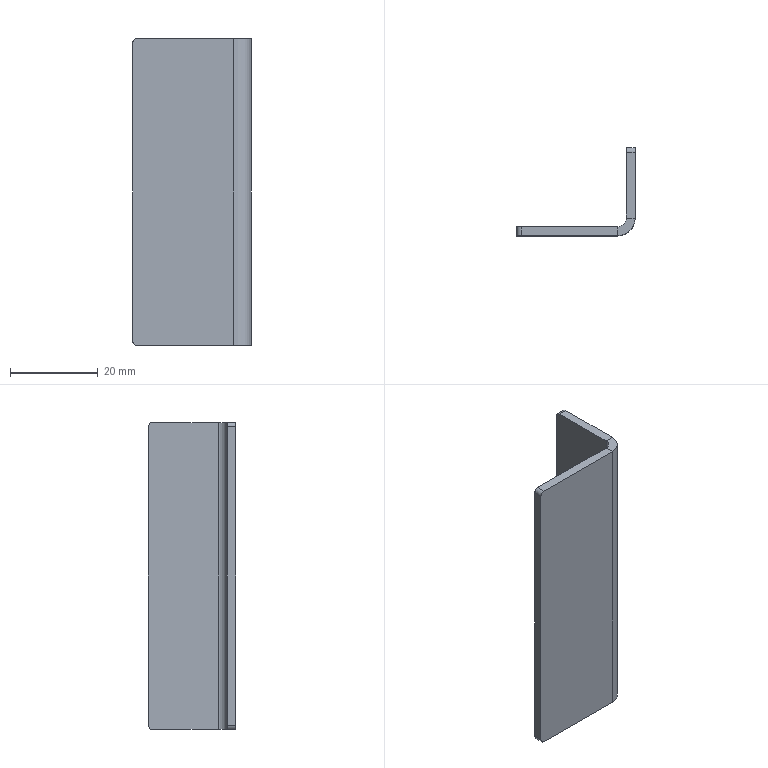Part | STEP file | 001-008-Traverse module detection sheet metal | 1 solid | 18 faces | box 27 x 20 x 70 mm | volume 6118 mm3 | plane 12 | cylinder 6 | commonest cylinder face diameters 2 x4 4 x1 8 x1
STEP:
#1=CARTESIAN_POINT('',(0.,0.,0.));
#2=DIRECTION('',(0.,0.,1.));
#3=DIRECTION('',(1.,0.,0.));
#4=AXIS2_PLACEMENT_3D('',#1,#2,#3);
#5=CARTESIAN_POINT('',(-4.,0.,35.));
#6=VERTEX_POINT('',#5);
#7=CARTESIAN_POINT('',(-4.,2.,35.));
#8=VERTEX_POINT('',#7);
#9=CARTESIAN_POINT('',(-4.,0.,35.));
#10=DIRECTION('',(0.,1.,0.));
#11=VECTOR('',#10,1.);
#12=LINE('',#9,#11);
#13=CARTESIAN_POINT('',(-4.,0.,35.));
#14=DIRECTION('',(0.,0.,1.));
#15=DIRECTION('',(1.,0.,0.));
#16=AXIS2_PLACEMENT_3D('',#13,#14,#15);
#17=PLANE('',#16);
#18=CARTESIAN_POINT('',(0.,0.));
#19=DIRECTION('',(0.,1.));
#20=VECTOR('',#19,1.);
#21=LINE('',#18,#20);
#22=(GEOMETRIC_REPRESENTATION_CONTEXT(2)PARAMETRIC_REPRESENTATION_CONTEXT()REPRESENTATION_CONTEXT('',''));
#23=DEFINITIONAL_REPRESENTATION('',(#21),#22);
#24=PCURVE('',#17,#23);
#25=CARTESIAN_POINT('',(-2.,4.,35.));
#26=DIRECTION('',(0.,0.,1.));
#27=DIRECTION('',(1.,0.,0.));
#28=AXIS2_PLACEMENT_3D('',#25,#26,#27);
#29=PLANE('',#28);
#30=CARTESIAN_POINT('',(-2.,-4.));
#31=DIRECTION('',(0.,1.));
#32=VECTOR('',#31,1.);
#33=LINE('',#30,#32);
#34=(GEOMETRIC_REPRESENTATION_CONTEXT(2)PARAMETRIC_REPRESENTATION_CONTEXT()REPRESENTATION_CONTEXT('',''));
#35=DEFINITIONAL_REPRESENTATION('',(#33),#34);
#36=PCURVE('',#29,#35);
#37=SURFACE_CURVE('',#12,(#24,#36),.PCURVE_S1.);
#38=EDGE_CURVE('',#6,#8,#37,.T.);
#39=ORIENTED_EDGE('',*,*,#38,.F.);
#40=CARTESIAN_POINT('',(0.,4.,35.));
#41=VERTEX_POINT('',#40);
#42=CARTESIAN_POINT('',(-4.,4.,35.));
#43=DIRECTION('',(0.,0.,-1.));
#44=DIRECTION('',(1.,0.,0.));
#45=AXIS2_PLACEMENT_3D('',#42,#43,#44);
#46=CIRCLE('',#45,4.);
#47=CARTESIAN_POINT('',(4.,4.));
#48=CARTESIAN_POINT('',(4.,-2.928));
#49=CARTESIAN_POINT('',(-2.,0.5359));
#50=CARTESIAN_POINT('',(-8.,4.));
#51=CARTESIAN_POINT('',(-2.,7.464));
#52=CARTESIAN_POINT('',(4.,10.928));
#53=CARTESIAN_POINT('',(4.,4.));
#54=(BOUNDED_CURVE()B_SPLINE_CURVE(2,(#47,#48,#49,#50,#51,#52,#53),.UNSPECIFIED.,.T.,.F.)B_SPLINE_CURVE_WITH_KNOTS((1,2,2,2,2,1),(-2.094,0.,2.094,4.189,6.283,8.378),.UNSPECIFIED.)CURVE()GEOMETRIC_REPRESENTATION_ITEM()RATIONAL_B_SPLINE_CURVE((1.,0.5,1.,0.5,1.,0.5,1.))REPRESENTATION_ITEM(''));
#55=(GEOMETRIC_REPRESENTATION_CONTEXT(2)PARAMETRIC_REPRESENTATION_CONTEXT()REPRESENTATION_CONTEXT('',''));
#56=DEFINITIONAL_REPRESENTATION('',(#54),#55);
#57=PCURVE('',#17,#56);
#58=CARTESIAN_POINT('',(-4.,4.,35.));
#59=DIRECTION('',(0.,0.,-1.));
#60=DIRECTION('',(-1.,0.,0.));
#61=AXIS2_PLACEMENT_3D('',#58,#59,#60);
#62=CYLINDRICAL_SURFACE('',#61,4.);
#63=CARTESIAN_POINT('',(3.142,0.));
#64=DIRECTION('',(1.,0.));
#65=VECTOR('',#64,1.);
#66=LINE('',#63,#65);
#67=(GEOMETRIC_REPRESENTATION_CONTEXT(2)PARAMETRIC_REPRESENTATION_CONTEXT()REPRESENTATION_CONTEXT('',''));
#68=DEFINITIONAL_REPRESENTATION('',(#66),#67);
#69=PCURVE('',#62,#68);
#70=SURFACE_CURVE('',#46,(#57,#69),.PCURVE_S1.);
#71=EDGE_CURVE('',#41,#6,#70,.T.);
#72=ORIENTED_EDGE('',*,*,#71,.F.);
#73=CARTESIAN_POINT('',(-2.,4.,35.));
#74=VERTEX_POINT('',#73);
#75=CARTESIAN_POINT('',(-2.,4.,35.));
#76=DIRECTION('',(1.,0.,0.));
#77=VECTOR('',#76,1.);
#78=LINE('',#75,#77);
#79=CARTESIAN_POINT('',(2.,4.));
#80=DIRECTION('',(1.,0.));
#81=VECTOR('',#80,1.);
#82=LINE('',#79,#81);
#83=(GEOMETRIC_REPRESENTATION_CONTEXT(2)PARAMETRIC_REPRESENTATION_CONTEXT()REPRESENTATION_CONTEXT('',''));
#84=DEFINITIONAL_REPRESENTATION('',(#82),#83);
#85=PCURVE('',#17,#84);
#86=CARTESIAN_POINT('',(-4.,4.,35.));
#87=DIRECTION('',(0.,0.,1.));
#88=DIRECTION('',(1.,0.,0.));
#89=AXIS2_PLACEMENT_3D('',#86,#87,#88);
#90=PLANE('',#89);
#91=CARTESIAN_POINT('',(2.,0.));
#92=DIRECTION('',(1.,0.));
#93=VECTOR('',#92,1.);
#94=LINE('',#91,#93);
#95=(GEOMETRIC_REPRESENTATION_CONTEXT(2)PARAMETRIC_REPRESENTATION_CONTEXT()REPRESENTATION_CONTEXT('',''));
#96=DEFINITIONAL_REPRESENTATION('',(#94),#95);
#97=PCURVE('',#90,#96);
#98=SURFACE_CURVE('',#78,(#85,#97),.PCURVE_S1.);
#99=EDGE_CURVE('',#74,#41,#98,.T.);
#100=ORIENTED_EDGE('',*,*,#99,.F.);
#101=CARTESIAN_POINT('',(-4.,4.,35.));
#102=DIRECTION('',(0.,0.,-1.));
#103=DIRECTION('',(1.,0.,0.));
#104=AXIS2_PLACEMENT_3D('',#101,#102,#103);
#105=CIRCLE('',#104,2.);
#106=CARTESIAN_POINT('',(2.,4.));
#107=CARTESIAN_POINT('',(2.,0.5359));
#108=CARTESIAN_POINT('',(-1.,2.268));
#109=CARTESIAN_POINT('',(-4.,4.));
#110=CARTESIAN_POINT('',(-1.,5.732));
#111=CARTESIAN_POINT('',(2.,7.464));
#112=CARTESIAN_POINT('',(2.,4.));
#113=(BOUNDED_CURVE()B_SPLINE_CURVE(2,(#106,#107,#108,#109,#110,#111,#112),.UNSPECIFIED.,.T.,.F.)B_SPLINE_CURVE_WITH_KNOTS((1,2,2,2,2,1),(-2.094,0.,2.094,4.189,6.283,8.378),.UNSPECIFIED.)CURVE()GEOMETRIC_REPRESENTATION_ITEM()RATIONAL_B_SPLINE_CURVE((1.,0.5,1.,0.5,1.,0.5,1.))REPRESENTATION_ITEM(''));
#114=(GEOMETRIC_REPRESENTATION_CONTEXT(2)PARAMETRIC_REPRESENTATION_CONTEXT()REPRESENTATION_CONTEXT('',''));
#115=DEFINITIONAL_REPRESENTATION('',(#113),#114);
#116=PCURVE('',#17,#115);
#117=CARTESIAN_POINT('',(-4.,4.,35.));
#118=DIRECTION('',(0.,0.,-1.));
#119=DIRECTION('',(-1.,0.,0.));
#120=AXIS2_PLACEMENT_3D('',#117,#118,#119);
#121=CYLINDRICAL_SURFACE('',#120,2.);
#122=CARTESIAN_POINT('',(3.142,0.));
#123=DIRECTION('',(1.,0.));
#124=VECTOR('',#123,1.);
#125=LINE('',#122,#124);
#126=(GEOMETRIC_REPRESENTATION_CONTEXT(2)PARAMETRIC_REPRESENTATION_CONTEXT()REPRESENTATION_CONTEXT('',''));
#127=DEFINITIONAL_REPRESENTATION('',(#125),#126);
#128=PCURVE('',#121,#127);
#129=SURFACE_CURVE('',#105,(#116,#128),.PCURVE_S1.);
#130=EDGE_CURVE('',#74,#8,#129,.T.);
#131=ORIENTED_EDGE('',*,*,#130,.T.);
#132=EDGE_LOOP('',(#39,#72,#100,#131));
#133=FACE_BOUND('',#132,.T.);
#134=ADVANCED_FACE('',(#133),#17,.T.);
#135=CARTESIAN_POINT('',(-26.,2.,35.));
#136=VERTEX_POINT('',#135);
#137=CARTESIAN_POINT('',(0.,2.,35.));
#138=DIRECTION('',(-1.,0.,0.));
#139=VECTOR('',#138,1.);
#140=LINE('',#137,#139);
#141=CARTESIAN_POINT('',(2.,-2.));
#142=DIRECTION('',(-1.,0.));
#143=VECTOR('',#142,1.);
#144=LINE('',#141,#143);
#145=(GEOMETRIC_REPRESENTATION_CONTEXT(2)PARAMETRIC_REPRESENTATION_CONTEXT()REPRESENTATION_CONTEXT('',''));
#146=DEFINITIONAL_REPRESENTATION('',(#144),#145);
#147=PCURVE('',#29,#146);
#148=CARTESIAN_POINT('',(0.,2.,35.));
#149=DIRECTION('',(0.,-1.,0.));
#150=DIRECTION('',(1.,0.,0.));
#151=AXIS2_PLACEMENT_3D('',#148,#149,#150);
#152=PLANE('',#151);
#153=CARTESIAN_POINT('',(0.,0.));
#154=DIRECTION('',(-1.,0.));
#155=VECTOR('',#154,1.);
#156=LINE('',#153,#155);
#157=(GEOMETRIC_REPRESENTATION_CONTEXT(2)PARAMETRIC_REPRESENTATION_CONTEXT()REPRESENTATION_CONTEXT('',''));
#158=DEFINITIONAL_REPRESENTATION('',(#156),#157);
#159=PCURVE('',#152,#158);
#160=SURFACE_CURVE('',#140,(#147,#159),.PCURVE_S1.);
#161=EDGE_CURVE('',#8,#136,#160,.T.);
#162=ORIENTED_EDGE('',*,*,#161,.T.);
#163=CARTESIAN_POINT('',(-26.,0.,35.));
#164=VERTEX_POINT('',#163);
#165=CARTESIAN_POINT('',(-26.,4.,35.));
#166=DIRECTION('',(0.,-1.,0.));
#167=VECTOR('',#166,1.);
#168=LINE('',#165,#167);
#169=CARTESIAN_POINT('',(-24.,0.));
#170=DIRECTION('',(0.,-1.));
#171=VECTOR('',#170,1.);
#172=LINE('',#169,#171);
#173=(GEOMETRIC_REPRESENTATION_CONTEXT(2)PARAMETRIC_REPRESENTATION_CONTEXT()REPRESENTATION_CONTEXT('',''));
#174=DEFINITIONAL_REPRESENTATION('',(#172),#173);
#175=PCURVE('',#29,#174);
#176=CARTESIAN_POINT('',(-26.,0.,34.));
#177=DIRECTION('',(0.,1.,0.));
#178=DIRECTION('',(0.,0.,1.));
#179=AXIS2_PLACEMENT_3D('',#176,#177,#178);
#180=CYLINDRICAL_SURFACE('',#179,1.);
#181=CARTESIAN_POINT('',(6.283,4.));
#182=DIRECTION('',(0.,-1.));
#183=VECTOR('',#182,1.);
#184=LINE('',#181,#183);
#185=(GEOMETRIC_REPRESENTATION_CONTEXT(2)PARAMETRIC_REPRESENTATION_CONTEXT()REPRESENTATION_CONTEXT('',''));
#186=DEFINITIONAL_REPRESENTATION('',(#184),#185);
#187=PCURVE('',#180,#186);
#188=SURFACE_CURVE('',#168,(#175,#187),.PCURVE_S1.);
#189=EDGE_CURVE('',#136,#164,#188,.T.);
#190=ORIENTED_EDGE('',*,*,#189,.T.);
#191=CARTESIAN_POINT('',(0.,0.,35.));
#192=DIRECTION('',(-1.,0.,0.));
#193=VECTOR('',#192,1.);
#194=LINE('',#191,#193);
#195=CARTESIAN_POINT('',(2.,-4.));
#196=DIRECTION('',(-1.,0.));
#197=VECTOR('',#196,1.);
#198=LINE('',#195,#197);
#199=(GEOMETRIC_REPRESENTATION_CONTEXT(2)PARAMETRIC_REPRESENTATION_CONTEXT()REPRESENTATION_CONTEXT('',''));
#200=DEFINITIONAL_REPRESENTATION('',(#198),#199);
#201=PCURVE('',#29,#200);
#202=CARTESIAN_POINT('',(0.,0.,35.));
#203=DIRECTION('',(0.,-1.,0.));
#204=DIRECTION('',(1.,0.,0.));
#205=AXIS2_PLACEMENT_3D('',#202,#203,#204);
#206=PLANE('',#205);
#207=CARTESIAN_POINT('',(0.,0.));
#208=DIRECTION('',(-1.,0.));
#209=VECTOR('',#208,1.);
#210=LINE('',#207,#209);
#211=(GEOMETRIC_REPRESENTATION_CONTEXT(2)PARAMETRIC_REPRESENTATION_CONTEXT()REPRESENTATION_CONTEXT('',''));
#212=DEFINITIONAL_REPRESENTATION('',(#210),#211);
#213=PCURVE('',#206,#212);
#214=SURFACE_CURVE('',#194,(#201,#213),.PCURVE_S1.);
#215=EDGE_CURVE('',#6,#164,#214,.T.);
#216=ORIENTED_EDGE('',*,*,#215,.F.);
#217=ORIENTED_EDGE('',*,*,#38,.T.);
#218=EDGE_LOOP('',(#162,#190,#216,#217));
#219=FACE_BOUND('',#218,.T.);
#220=ADVANCED_FACE('',(#219),#29,.T.);
#221=CARTESIAN_POINT('',(0.,4.,-35.));
#222=VERTEX_POINT('',#221);
#223=CARTESIAN_POINT('',(-2.,4.,-35.));
#224=VERTEX_POINT('',#223);
#225=CARTESIAN_POINT('',(0.,4.,-35.));
#226=DIRECTION('',(-1.,0.,0.));
#227=VECTOR('',#226,1.);
#228=LINE('',#225,#227);
#229=CARTESIAN_POINT('',(0.,4.,-35.));
#230=DIRECTION('',(0.,0.,-1.));
#231=DIRECTION('',(-1.,0.,0.));
#232=AXIS2_PLACEMENT_3D('',#229,#230,#231);
#233=PLANE('',#232);
#234=CARTESIAN_POINT('',(0.,0.));
#235=DIRECTION('',(1.,0.));
#236=VECTOR('',#235,1.);
#237=LINE('',#234,#236);
#238=(GEOMETRIC_REPRESENTATION_CONTEXT(2)PARAMETRIC_REPRESENTATION_CONTEXT()REPRESENTATION_CONTEXT('',''));
#239=DEFINITIONAL_REPRESENTATION('',(#237),#238);
#240=PCURVE('',#233,#239);
#241=CARTESIAN_POINT('',(-4.,2.,-35.));
#242=DIRECTION('',(0.,0.,-1.));
#243=DIRECTION('',(-1.,0.,0.));
#244=AXIS2_PLACEMENT_3D('',#241,#242,#243);
#245=PLANE('',#244);
#246=CARTESIAN_POINT('',(-4.,2.));
#247=DIRECTION('',(1.,0.));
#248=VECTOR('',#247,1.);
#249=LINE('',#246,#248);
#250=(GEOMETRIC_REPRESENTATION_CONTEXT(2)PARAMETRIC_REPRESENTATION_CONTEXT()REPRESENTATION_CONTEXT('',''));
#251=DEFINITIONAL_REPRESENTATION('',(#249),#250);
#252=PCURVE('',#245,#251);
#253=SURFACE_CURVE('',#228,(#240,#252),.PCURVE_S1.);
#254=EDGE_CURVE('',#222,#224,#253,.T.);
#255=ORIENTED_EDGE('',*,*,#254,.F.);
#256=CARTESIAN_POINT('',(-4.,0.,-35.));
#257=VERTEX_POINT('',#256);
#258=CARTESIAN_POINT('',(-4.,4.,-35.));
#259=DIRECTION('',(0.,0.,-1.));
#260=DIRECTION('',(1.,0.,0.));
#261=AXIS2_PLACEMENT_3D('',#258,#259,#260);
#262=CIRCLE('',#261,4.);
#263=CARTESIAN_POINT('',(4.,0.));
#264=DIRECTION('',(-1.,0.));
#265=AXIS2_PLACEMENT_2D('',#263,#264);
#266=CIRCLE('',#265,4.);
#267=(GEOMETRIC_REPRESENTATION_CONTEXT(2)PARAMETRIC_REPRESENTATION_CONTEXT()REPRESENTATION_CONTEXT('',''));
#268=DEFINITIONAL_REPRESENTATION('',(#266),#267);
#269=PCURVE('',#233,#268);
#270=CARTESIAN_POINT('',(3.142,70.));
#271=DIRECTION('',(1.,0.));
#272=VECTOR('',#271,1.);
#273=LINE('',#270,#272);
#274=(GEOMETRIC_REPRESENTATION_CONTEXT(2)PARAMETRIC_REPRESENTATION_CONTEXT()REPRESENTATION_CONTEXT('',''));
#275=DEFINITIONAL_REPRESENTATION('',(#273),#274);
#276=PCURVE('',#62,#275);
#277=SURFACE_CURVE('',#262,(#269,#276),.PCURVE_S1.);
#278=EDGE_CURVE('',#222,#257,#277,.T.);
#279=ORIENTED_EDGE('',*,*,#278,.T.);
#280=CARTESIAN_POINT('',(-4.,2.,-35.));
#281=VERTEX_POINT('',#280);
#282=CARTESIAN_POINT('',(-4.,2.,-35.));
#283=DIRECTION('',(0.,-1.,0.));
#284=VECTOR('',#283,1.);
#285=LINE('',#282,#284);
#286=CARTESIAN_POINT('',(4.,-2.));
#287=DIRECTION('',(0.,-1.));
#288=VECTOR('',#287,1.);
#289=LINE('',#286,#288);
#290=(GEOMETRIC_REPRESENTATION_CONTEXT(2)PARAMETRIC_REPRESENTATION_CONTEXT()REPRESENTATION_CONTEXT('',''));
#291=DEFINITIONAL_REPRESENTATION('',(#289),#290);
#292=PCURVE('',#233,#291);
#293=CARTESIAN_POINT('',(-4.,4.,-35.));
#294=DIRECTION('',(0.,0.,1.));
#295=DIRECTION('',(1.,0.,0.));
#296=AXIS2_PLACEMENT_3D('',#293,#294,#295);
#297=PLANE('',#296);
#298=CARTESIAN_POINT('',(0.,-2.));
#299=DIRECTION('',(0.,-1.));
#300=VECTOR('',#299,1.);
#301=LINE('',#298,#300);
#302=(GEOMETRIC_REPRESENTATION_CONTEXT(2)PARAMETRIC_REPRESENTATION_CONTEXT()REPRESENTATION_CONTEXT('',''));
#303=DEFINITIONAL_REPRESENTATION('',(#301),#302);
#304=PCURVE('',#297,#303);
#305=SURFACE_CURVE('',#285,(#292,#304),.PCURVE_S1.);
#306=EDGE_CURVE('',#281,#257,#305,.T.);
#307=ORIENTED_EDGE('',*,*,#306,.F.);
#308=CARTESIAN_POINT('',(-4.,4.,-35.));
#309=DIRECTION('',(0.,0.,-1.));
#310=DIRECTION('',(1.,0.,0.));
#311=AXIS2_PLACEMENT_3D('',#308,#309,#310);
#312=CIRCLE('',#311,2.);
#313=CARTESIAN_POINT('',(4.,0.));
#314=DIRECTION('',(-1.,0.));
#315=AXIS2_PLACEMENT_2D('',#313,#314);
#316=CIRCLE('',#315,2.);
#317=(GEOMETRIC_REPRESENTATION_CONTEXT(2)PARAMETRIC_REPRESENTATION_CONTEXT()REPRESENTATION_CONTEXT('',''));
#318=DEFINITIONAL_REPRESENTATION('',(#316),#317);
#319=PCURVE('',#233,#318);
#320=CARTESIAN_POINT('',(3.142,70.));
#321=DIRECTION('',(1.,0.));
#322=VECTOR('',#321,1.);
#323=LINE('',#320,#322);
#324=(GEOMETRIC_REPRESENTATION_CONTEXT(2)PARAMETRIC_REPRESENTATION_CONTEXT()REPRESENTATION_CONTEXT('',''));
#325=DEFINITIONAL_REPRESENTATION('',(#323),#324);
#326=PCURVE('',#121,#325);
#327=SURFACE_CURVE('',#312,(#319,#326),.PCURVE_S1.);
#328=EDGE_CURVE('',#224,#281,#327,.T.);
#329=ORIENTED_EDGE('',*,*,#328,.F.);
#330=EDGE_LOOP('',(#255,#279,#307,#329));
#331=FACE_BOUND('',#330,.T.);
#332=ADVANCED_FACE('',(#331),#233,.T.);
#333=CARTESIAN_POINT('',(-2.,19.,-35.));
#334=VERTEX_POINT('',#333);
#335=CARTESIAN_POINT('',(-2.,0.,-35.));
#336=DIRECTION('',(0.,-1.,0.));
#337=VECTOR('',#336,1.);
#338=LINE('',#335,#337);
#339=CARTESIAN_POINT('',(-2.,-2.));
#340=DIRECTION('',(0.,-1.));
#341=VECTOR('',#340,1.);
#342=LINE('',#339,#341);
#343=(GEOMETRIC_REPRESENTATION_CONTEXT(2)PARAMETRIC_REPRESENTATION_CONTEXT()REPRESENTATION_CONTEXT('',''));
#344=DEFINITIONAL_REPRESENTATION('',(#342),#343);
#345=PCURVE('',#245,#344);
#346=CARTESIAN_POINT('',(-2.,0.,35.));
#347=DIRECTION('',(1.,0.,0.));
#348=DIRECTION('',(0.,0.,-1.));
#349=AXIS2_PLACEMENT_3D('',#346,#347,#348);
#350=PLANE('',#349);
#351=CARTESIAN_POINT('',(70.,0.));
#352=DIRECTION('',(0.,-1.));
#353=VECTOR('',#352,1.);
#354=LINE('',#351,#353);
#355=(GEOMETRIC_REPRESENTATION_CONTEXT(2)PARAMETRIC_REPRESENTATION_CONTEXT()REPRESENTATION_CONTEXT('',''));
#356=DEFINITIONAL_REPRESENTATION('',(#354),#355);
#357=PCURVE('',#350,#356);
#358=SURFACE_CURVE('',#338,(#345,#357),.PCURVE_S1.);
#359=EDGE_CURVE('',#334,#224,#358,.T.);
#360=ORIENTED_EDGE('',*,*,#359,.F.);
#361=CARTESIAN_POINT('',(0.,19.,-35.));
#362=VERTEX_POINT('',#361);
#363=CARTESIAN_POINT('',(-4.,19.,-35.));
#364=DIRECTION('',(1.,0.,0.));
#365=VECTOR('',#364,1.);
#366=LINE('',#363,#365);
#367=CARTESIAN_POINT('',(0.,17.));
#368=DIRECTION('',(-1.,0.));
#369=VECTOR('',#368,1.);
#370=LINE('',#367,#369);
#371=(GEOMETRIC_REPRESENTATION_CONTEXT(2)PARAMETRIC_REPRESENTATION_CONTEXT()REPRESENTATION_CONTEXT('',''));
#372=DEFINITIONAL_REPRESENTATION('',(#370),#371);
#373=PCURVE('',#245,#372);
#374=CARTESIAN_POINT('',(-4.,19.,-34.));
#375=DIRECTION('',(1.,0.,0.));
#376=DIRECTION('',(0.,0.,-1.));
#377=AXIS2_PLACEMENT_3D('',#374,#375,#376);
#378=CYLINDRICAL_SURFACE('',#377,1.);
#379=CARTESIAN_POINT('',(0.,0.));
#380=DIRECTION('',(0.,1.));
#381=VECTOR('',#380,1.);
#382=LINE('',#379,#381);
#383=(GEOMETRIC_REPRESENTATION_CONTEXT(2)PARAMETRIC_REPRESENTATION_CONTEXT()REPRESENTATION_CONTEXT('',''));
#384=DEFINITIONAL_REPRESENTATION('',(#382),#383);
#385=PCURVE('',#378,#384);
#386=SURFACE_CURVE('',#366,(#373,#385),.PCURVE_S1.);
#387=EDGE_CURVE('',#334,#362,#386,.T.);
#388=ORIENTED_EDGE('',*,*,#387,.T.);
#389=CARTESIAN_POINT('',(0.,0.,-35.));
#390=DIRECTION('',(0.,-1.,0.));
#391=VECTOR('',#390,1.);
#392=LINE('',#389,#391);
#393=CARTESIAN_POINT('',(-4.,-2.));
#394=DIRECTION('',(0.,-1.));
#395=VECTOR('',#394,1.);
#396=LINE('',#393,#395);
#397=(GEOMETRIC_REPRESENTATION_CONTEXT(2)PARAMETRIC_REPRESENTATION_CONTEXT()REPRESENTATION_CONTEXT('',''));
#398=DEFINITIONAL_REPRESENTATION('',(#396),#397);
#399=PCURVE('',#245,#398);
#400=CARTESIAN_POINT('',(0.,0.,35.));
#401=DIRECTION('',(1.,0.,0.));
#402=DIRECTION('',(0.,0.,-1.));
#403=AXIS2_PLACEMENT_3D('',#400,#401,#402);
#404=PLANE('',#403);
#405=CARTESIAN_POINT('',(70.,0.));
#406=DIRECTION('',(0.,-1.));
#407=VECTOR('',#406,1.);
#408=LINE('',#405,#407);
#409=(GEOMETRIC_REPRESENTATION_CONTEXT(2)PARAMETRIC_REPRESENTATION_CONTEXT()REPRESENTATION_CONTEXT('',''));
#410=DEFINITIONAL_REPRESENTATION('',(#408),#409);
#411=PCURVE('',#404,#410);
#412=SURFACE_CURVE('',#392,(#399,#411),.PCURVE_S1.);
#413=EDGE_CURVE('',#362,#222,#412,.T.);
#414=ORIENTED_EDGE('',*,*,#413,.T.);
#415=ORIENTED_EDGE('',*,*,#254,.T.);
#416=EDGE_LOOP('',(#360,#388,#414,#415));
#417=FACE_BOUND('',#416,.T.);
#418=ADVANCED_FACE('',(#417),#245,.T.);
#419=CARTESIAN_POINT('',(-27.,2.,34.));
#420=VERTEX_POINT('',#419);
#421=CARTESIAN_POINT('',(-27.,2.,-34.));
#422=VERTEX_POINT('',#421);
#423=CARTESIAN_POINT('',(-27.,2.,35.));
#424=DIRECTION('',(0.,0.,-1.));
#425=VECTOR('',#424,1.);
#426=LINE('',#423,#425);
#427=CARTESIAN_POINT('',(-27.,0.));
#428=DIRECTION('',(0.,-1.));
#429=VECTOR('',#428,1.);
#430=LINE('',#427,#429);
#431=(GEOMETRIC_REPRESENTATION_CONTEXT(2)PARAMETRIC_REPRESENTATION_CONTEXT()REPRESENTATION_CONTEXT('',''));
#432=DEFINITIONAL_REPRESENTATION('',(#430),#431);
#433=PCURVE('',#152,#432);
#434=CARTESIAN_POINT('',(-27.,0.,35.));
#435=DIRECTION('',(-1.,0.,0.));
#436=DIRECTION('',(0.,0.,1.));
#437=AXIS2_PLACEMENT_3D('',#434,#435,#436);
#438=PLANE('',#437);
#439=CARTESIAN_POINT('',(0.,2.));
#440=DIRECTION('',(-1.,0.));
#441=VECTOR('',#440,1.);
#442=LINE('',#439,#441);
#443=(GEOMETRIC_REPRESENTATION_CONTEXT(2)PARAMETRIC_REPRESENTATION_CONTEXT()REPRESENTATION_CONTEXT('',''));
#444=DEFINITIONAL_REPRESENTATION('',(#442),#443);
#445=PCURVE('',#438,#444);
#446=SURFACE_CURVE('',#426,(#433,#445),.PCURVE_S1.);
#447=EDGE_CURVE('',#420,#422,#446,.T.);
#448=ORIENTED_EDGE('',*,*,#447,.F.);
#449=CARTESIAN_POINT('',(-26.,2.,34.));
#450=DIRECTION('',(0.,1.,0.));
#451=DIRECTION('',(1.,0.,0.));
#452=AXIS2_PLACEMENT_3D('',#449,#450,#451);
#453=CIRCLE('',#452,1.);
#454=CARTESIAN_POINT('',(-25.,-1.));
#455=CARTESIAN_POINT('',(-25.,-2.732));
#456=CARTESIAN_POINT('',(-26.5,-1.866));
#457=CARTESIAN_POINT('',(-28.,-1.));
#458=CARTESIAN_POINT('',(-26.5,-0.134));
#459=CARTESIAN_POINT('',(-25.,0.7321));
#460=CARTESIAN_POINT('',(-25.,-1.));
#461=(BOUNDED_CURVE()B_SPLINE_CURVE(2,(#454,#455,#456,#457,#458,#459,#460),.UNSPECIFIED.,.T.,.F.)B_SPLINE_CURVE_WITH_KNOTS((1,2,2,2,2,1),(-2.094,0.,2.094,4.189,6.283,8.378),.UNSPECIFIED.)CURVE()GEOMETRIC_REPRESENTATION_ITEM()RATIONAL_B_SPLINE_CURVE((1.,0.5,1.,0.5,1.,0.5,1.))REPRESENTATION_ITEM(''));
#462=(GEOMETRIC_REPRESENTATION_CONTEXT(2)PARAMETRIC_REPRESENTATION_CONTEXT()REPRESENTATION_CONTEXT('',''));
#463=DEFINITIONAL_REPRESENTATION('',(#461),#462);
#464=PCURVE('',#152,#463);
#465=CARTESIAN_POINT('',(1.571,2.));
#466=DIRECTION('',(1.,0.));
#467=VECTOR('',#466,1.);
#468=LINE('',#465,#467);
#469=(GEOMETRIC_REPRESENTATION_CONTEXT(2)PARAMETRIC_REPRESENTATION_CONTEXT()REPRESENTATION_CONTEXT('',''));
#470=DEFINITIONAL_REPRESENTATION('',(#468),#469);
#471=PCURVE('',#180,#470);
#472=SURFACE_CURVE('',#453,(#464,#471),.PCURVE_S1.);
#473=EDGE_CURVE('',#420,#136,#472,.T.);
#474=ORIENTED_EDGE('',*,*,#473,.T.);
#475=ORIENTED_EDGE('',*,*,#161,.F.);
#476=CARTESIAN_POINT('',(-4.,2.,35.));
#477=DIRECTION('',(0.,0.,-1.));
#478=VECTOR('',#477,1.);
#479=LINE('',#476,#478);
#480=CARTESIAN_POINT('',(-4.,0.));
#481=DIRECTION('',(0.,-1.));
#482=VECTOR('',#481,1.);
#483=LINE('',#480,#482);
#484=(GEOMETRIC_REPRESENTATION_CONTEXT(2)PARAMETRIC_REPRESENTATION_CONTEXT()REPRESENTATION_CONTEXT('',''));
#485=DEFINITIONAL_REPRESENTATION('',(#483),#484);
#486=PCURVE('',#152,#485);
#487=CARTESIAN_POINT('',(4.712,0.));
#488=DIRECTION('',(0.,1.));
#489=VECTOR('',#488,1.);
#490=LINE('',#487,#489);
#491=(GEOMETRIC_REPRESENTATION_CONTEXT(2)PARAMETRIC_REPRESENTATION_CONTEXT()REPRESENTATION_CONTEXT('',''));
#492=DEFINITIONAL_REPRESENTATION('',(#490),#491);
#493=PCURVE('',#121,#492);
#494=SURFACE_CURVE('',#479,(#486,#493),.PCURVE_S1.);
#495=EDGE_CURVE('',#8,#281,#494,.T.);
#496=ORIENTED_EDGE('',*,*,#495,.T.);
#497=CARTESIAN_POINT('',(-26.,2.,-35.));
#498=VERTEX_POINT('',#497);
#499=CARTESIAN_POINT('',(0.,2.,-35.));
#500=DIRECTION('',(-1.,0.,0.));
#501=VECTOR('',#500,1.);
#502=LINE('',#499,#501);
#503=CARTESIAN_POINT('',(0.,-70.));
#504=DIRECTION('',(-1.,0.));
#505=VECTOR('',#504,1.);
#506=LINE('',#503,#505);
#507=(GEOMETRIC_REPRESENTATION_CONTEXT(2)PARAMETRIC_REPRESENTATION_CONTEXT()REPRESENTATION_CONTEXT('',''));
#508=DEFINITIONAL_REPRESENTATION('',(#506),#507);
#509=PCURVE('',#152,#508);
#510=CARTESIAN_POINT('',(4.,-2.));
#511=DIRECTION('',(-1.,0.));
#512=VECTOR('',#511,1.);
#513=LINE('',#510,#512);
#514=(GEOMETRIC_REPRESENTATION_CONTEXT(2)PARAMETRIC_REPRESENTATION_CONTEXT()REPRESENTATION_CONTEXT('',''));
#515=DEFINITIONAL_REPRESENTATION('',(#513),#514);
#516=PCURVE('',#297,#515);
#517=SURFACE_CURVE('',#502,(#509,#516),.PCURVE_S1.);
#518=EDGE_CURVE('',#281,#498,#517,.T.);
#519=ORIENTED_EDGE('',*,*,#518,.T.);
#520=CARTESIAN_POINT('',(-26.,2.,-34.));
#521=DIRECTION('',(0.,1.,0.));
#522=DIRECTION('',(1.,0.,0.));
#523=AXIS2_PLACEMENT_3D('',#520,#521,#522);
#524=CIRCLE('',#523,1.);
#525=CARTESIAN_POINT('',(-25.,-69.));
#526=CARTESIAN_POINT('',(-25.,-70.732));
#527=CARTESIAN_POINT('',(-26.5,-69.866));
#528=CARTESIAN_POINT('',(-28.,-69.));
#529=CARTESIAN_POINT('',(-26.5,-68.134));
#530=CARTESIAN_POINT('',(-25.,-67.268));
#531=CARTESIAN_POINT('',(-25.,-69.));
#532=(BOUNDED_CURVE()B_SPLINE_CURVE(2,(#525,#526,#527,#528,#529,#530,#531),.UNSPECIFIED.,.T.,.F.)B_SPLINE_CURVE_WITH_KNOTS((1,2,2,2,2,1),(-2.094,0.,2.094,4.189,6.283,8.378),.UNSPECIFIED.)CURVE()GEOMETRIC_REPRESENTATION_ITEM()RATIONAL_B_SPLINE_CURVE((1.,0.5,1.,0.5,1.,0.5,1.))REPRESENTATION_ITEM(''));
#533=(GEOMETRIC_REPRESENTATION_CONTEXT(2)PARAMETRIC_REPRESENTATION_CONTEXT()REPRESENTATION_CONTEXT('',''));
#534=DEFINITIONAL_REPRESENTATION('',(#532),#533);
#535=PCURVE('',#152,#534);
#536=CARTESIAN_POINT('',(-26.,4.,-34.));
#537=DIRECTION('',(0.,-1.,0.));
#538=DIRECTION('',(0.,0.,-1.));
#539=AXIS2_PLACEMENT_3D('',#536,#537,#538);
#540=CYLINDRICAL_SURFACE('',#539,1.);
#541=CARTESIAN_POINT('',(7.854,2.));
#542=DIRECTION('',(-1.,0.));
#543=VECTOR('',#542,1.);
#544=LINE('',#541,#543);
#545=(GEOMETRIC_REPRESENTATION_CONTEXT(2)PARAMETRIC_REPRESENTATION_CONTEXT()REPRESENTATION_CONTEXT('',''));
#546=DEFINITIONAL_REPRESENTATION('',(#544),#545);
#547=PCURVE('',#540,#546);
#548=SURFACE_CURVE('',#524,(#535,#547),.PCURVE_S1.);
#549=EDGE_CURVE('',#498,#422,#548,.T.);
#550=ORIENTED_EDGE('',*,*,#549,.T.);
#551=EDGE_LOOP('',(#448,#474,#475,#496,#519,#550));
#552=FACE_BOUND('',#551,.T.);
#553=ADVANCED_FACE('',(#552),#152,.F.);
#554=CARTESIAN_POINT('',(-27.,0.,34.));
#555=VERTEX_POINT('',#554);
#556=CARTESIAN_POINT('',(-27.,0.,-34.));
#557=VERTEX_POINT('',#556);
#558=CARTESIAN_POINT('',(-27.,0.,35.));
#559=DIRECTION('',(0.,0.,-1.));
#560=VECTOR('',#559,1.);
#561=LINE('',#558,#560);
#562=CARTESIAN_POINT('',(0.,0.));
#563=DIRECTION('',(-1.,0.));
#564=VECTOR('',#563,1.);
#565=LINE('',#562,#564);
#566=(GEOMETRIC_REPRESENTATION_CONTEXT(2)PARAMETRIC_REPRESENTATION_CONTEXT()REPRESENTATION_CONTEXT('',''));
#567=DEFINITIONAL_REPRESENTATION('',(#565),#566);
#568=PCURVE('',#438,#567);
#569=CARTESIAN_POINT('',(-27.,0.));
#570=DIRECTION('',(0.,-1.));
#571=VECTOR('',#570,1.);
#572=LINE('',#569,#571);
#573=(GEOMETRIC_REPRESENTATION_CONTEXT(2)PARAMETRIC_REPRESENTATION_CONTEXT()REPRESENTATION_CONTEXT('',''));
#574=DEFINITIONAL_REPRESENTATION('',(#572),#573);
#575=PCURVE('',#206,#574);
#576=SURFACE_CURVE('',#561,(#568,#575),.PCURVE_S1.);
#577=EDGE_CURVE('',#555,#557,#576,.T.);
#578=ORIENTED_EDGE('',*,*,#577,.F.);
#579=CARTESIAN_POINT('',(-27.,0.,34.));
#580=DIRECTION('',(0.,1.,0.));
#581=VECTOR('',#580,1.);
#582=LINE('',#579,#581);
#583=CARTESIAN_POINT('',(-1.,0.));
#584=DIRECTION('',(0.,1.));
#585=VECTOR('',#584,1.);
#586=LINE('',#583,#585);
#587=(GEOMETRIC_REPRESENTATION_CONTEXT(2)PARAMETRIC_REPRESENTATION_CONTEXT()REPRESENTATION_CONTEXT('',''));
#588=DEFINITIONAL_REPRESENTATION('',(#586),#587);
#589=PCURVE('',#438,#588);
#590=CARTESIAN_POINT('',(4.712,0.));
#591=DIRECTION('',(0.,1.));
#592=VECTOR('',#591,1.);
#593=LINE('',#590,#592);
#594=(GEOMETRIC_REPRESENTATION_CONTEXT(2)PARAMETRIC_REPRESENTATION_CONTEXT()REPRESENTATION_CONTEXT('',''));
#595=DEFINITIONAL_REPRESENTATION('',(#593),#594);
#596=PCURVE('',#180,#595);
#597=SURFACE_CURVE('',#582,(#589,#596),.PCURVE_S1.);
#598=EDGE_CURVE('',#555,#420,#597,.T.);
#599=ORIENTED_EDGE('',*,*,#598,.T.);
#600=ORIENTED_EDGE('',*,*,#447,.T.);
#601=CARTESIAN_POINT('',(-27.,0.,-34.));
#602=DIRECTION('',(0.,-1.,0.));
#603=VECTOR('',#602,1.);
#604=LINE('',#601,#603);
#605=CARTESIAN_POINT('',(-69.,0.));
#606=DIRECTION('',(0.,-1.));
#607=VECTOR('',#606,1.);
#608=LINE('',#605,#607);
#609=(GEOMETRIC_REPRESENTATION_CONTEXT(2)PARAMETRIC_REPRESENTATION_CONTEXT()REPRESENTATION_CONTEXT('',''));
#610=DEFINITIONAL_REPRESENTATION('',(#608),#609);
#611=PCURVE('',#438,#610);
#612=CARTESIAN_POINT('',(4.712,4.));
#613=DIRECTION('',(0.,1.));
#614=VECTOR('',#613,1.);
#615=LINE('',#612,#614);
#616=(GEOMETRIC_REPRESENTATION_CONTEXT(2)PARAMETRIC_REPRESENTATION_CONTEXT()REPRESENTATION_CONTEXT('',''));
#617=DEFINITIONAL_REPRESENTATION('',(#615),#616);
#618=PCURVE('',#540,#617);
#619=SURFACE_CURVE('',#604,(#611,#618),.PCURVE_S1.);
#620=EDGE_CURVE('',#422,#557,#619,.T.);
#621=ORIENTED_EDGE('',*,*,#620,.T.);
#622=EDGE_LOOP('',(#578,#599,#600,#621));
#623=FACE_BOUND('',#622,.T.);
#624=ADVANCED_FACE('',(#623),#438,.T.);
#625=ORIENTED_EDGE('',*,*,#215,.T.);
#626=CARTESIAN_POINT('',(-26.,0.,34.));
#627=DIRECTION('',(0.,-1.,0.));
#628=DIRECTION('',(1.,0.,0.));
#629=AXIS2_PLACEMENT_3D('',#626,#627,#628);
#630=CIRCLE('',#629,1.);
#631=CARTESIAN_POINT('',(-26.,-1.));
#632=DIRECTION('',(1.,0.));
#633=AXIS2_PLACEMENT_2D('',#631,#632);
#634=CIRCLE('',#633,1.);
#635=(GEOMETRIC_REPRESENTATION_CONTEXT(2)PARAMETRIC_REPRESENTATION_CONTEXT()REPRESENTATION_CONTEXT('',''));
#636=DEFINITIONAL_REPRESENTATION('',(#634),#635);
#637=PCURVE('',#206,#636);
#638=CARTESIAN_POINT('',(7.854,0.));
#639=DIRECTION('',(-1.,0.));
#640=VECTOR('',#639,1.);
#641=LINE('',#638,#640);
#642=(GEOMETRIC_REPRESENTATION_CONTEXT(2)PARAMETRIC_REPRESENTATION_CONTEXT()REPRESENTATION_CONTEXT('',''));
#643=DEFINITIONAL_REPRESENTATION('',(#641),#642);
#644=PCURVE('',#180,#643);
#645=SURFACE_CURVE('',#630,(#637,#644),.PCURVE_S1.);
#646=EDGE_CURVE('',#164,#555,#645,.T.);
#647=ORIENTED_EDGE('',*,*,#646,.T.);
#648=ORIENTED_EDGE('',*,*,#577,.T.);
#649=CARTESIAN_POINT('',(-26.,0.,-35.));
#650=VERTEX_POINT('',#649);
#651=CARTESIAN_POINT('',(-26.,0.,-34.));
#652=DIRECTION('',(0.,-1.,0.));
#653=DIRECTION('',(1.,0.,0.));
#654=AXIS2_PLACEMENT_3D('',#651,#652,#653);
#655=CIRCLE('',#654,1.);
#656=CARTESIAN_POINT('',(-26.,-69.));
#657=DIRECTION('',(1.,0.));
#658=AXIS2_PLACEMENT_2D('',#656,#657);
#659=CIRCLE('',#658,1.);
#660=(GEOMETRIC_REPRESENTATION_CONTEXT(2)PARAMETRIC_REPRESENTATION_CONTEXT()REPRESENTATION_CONTEXT('',''));
#661=DEFINITIONAL_REPRESENTATION('',(#659),#660);
#662=PCURVE('',#206,#661);
#663=CARTESIAN_POINT('',(1.571,4.));
#664=DIRECTION('',(1.,0.));
#665=VECTOR('',#664,1.);
#666=LINE('',#663,#665);
#667=(GEOMETRIC_REPRESENTATION_CONTEXT(2)PARAMETRIC_REPRESENTATION_CONTEXT()REPRESENTATION_CONTEXT('',''));
#668=DEFINITIONAL_REPRESENTATION('',(#666),#667);
#669=PCURVE('',#540,#668);
#670=SURFACE_CURVE('',#655,(#662,#669),.PCURVE_S1.);
#671=EDGE_CURVE('',#557,#650,#670,.T.);
#672=ORIENTED_EDGE('',*,*,#671,.T.);
#673=CARTESIAN_POINT('',(0.,0.,-35.));
#674=DIRECTION('',(-1.,0.,0.));
#675=VECTOR('',#674,1.);
#676=LINE('',#673,#675);
#677=CARTESIAN_POINT('',(0.,-70.));
#678=DIRECTION('',(-1.,0.));
#679=VECTOR('',#678,1.);
#680=LINE('',#677,#679);
#681=(GEOMETRIC_REPRESENTATION_CONTEXT(2)PARAMETRIC_REPRESENTATION_CONTEXT()REPRESENTATION_CONTEXT('',''));
#682=DEFINITIONAL_REPRESENTATION('',(#680),#681);
#683=PCURVE('',#206,#682);
#684=CARTESIAN_POINT('',(4.,-4.));
#685=DIRECTION('',(-1.,0.));
#686=VECTOR('',#685,1.);
#687=LINE('',#684,#686);
#688=(GEOMETRIC_REPRESENTATION_CONTEXT(2)PARAMETRIC_REPRESENTATION_CONTEXT()REPRESENTATION_CONTEXT('',''));
#689=DEFINITIONAL_REPRESENTATION('',(#687),#688);
#690=PCURVE('',#297,#689);
#691=SURFACE_CURVE('',#676,(#683,#690),.PCURVE_S1.);
#692=EDGE_CURVE('',#257,#650,#691,.T.);
#693=ORIENTED_EDGE('',*,*,#692,.F.);
#694=CARTESIAN_POINT('',(-4.,0.,35.));
#695=DIRECTION('',(0.,0.,-1.));
#696=VECTOR('',#695,1.);
#697=LINE('',#694,#696);
#698=CARTESIAN_POINT('',(-4.,0.));
#699=DIRECTION('',(0.,-1.));
#700=VECTOR('',#699,1.);
#701=LINE('',#698,#700);
#702=(GEOMETRIC_REPRESENTATION_CONTEXT(2)PARAMETRIC_REPRESENTATION_CONTEXT()REPRESENTATION_CONTEXT('',''));
#703=DEFINITIONAL_REPRESENTATION('',(#701),#702);
#704=PCURVE('',#206,#703);
#705=CARTESIAN_POINT('',(4.712,0.));
#706=DIRECTION('',(0.,1.));
#707=VECTOR('',#706,1.);
#708=LINE('',#705,#707);
#709=(GEOMETRIC_REPRESENTATION_CONTEXT(2)PARAMETRIC_REPRESENTATION_CONTEXT()REPRESENTATION_CONTEXT('',''));
#710=DEFINITIONAL_REPRESENTATION('',(#708),#709);
#711=PCURVE('',#62,#710);
#712=SURFACE_CURVE('',#697,(#704,#711),.PCURVE_S1.);
#713=EDGE_CURVE('',#6,#257,#712,.T.);
#714=ORIENTED_EDGE('',*,*,#713,.F.);
#715=EDGE_LOOP('',(#625,#647,#648,#672,#693,#714));
#716=FACE_BOUND('',#715,.T.);
#717=ADVANCED_FACE('',(#716),#206,.T.);
#718=ORIENTED_EDGE('',*,*,#278,.F.);
#719=CARTESIAN_POINT('',(0.,4.,35.));
#720=DIRECTION('',(0.,0.,-1.));
#721=VECTOR('',#720,1.);
#722=LINE('',#719,#721);
#723=CARTESIAN_POINT('',(3.142,0.));
#724=DIRECTION('',(0.,1.));
#725=VECTOR('',#724,1.);
#726=LINE('',#723,#725);
#727=(GEOMETRIC_REPRESENTATION_CONTEXT(2)PARAMETRIC_REPRESENTATION_CONTEXT()REPRESENTATION_CONTEXT('',''));
#728=DEFINITIONAL_REPRESENTATION('',(#726),#727);
#729=PCURVE('',#62,#728);
#730=CARTESIAN_POINT('',(0.,4.));
#731=DIRECTION('',(1.,0.));
#732=VECTOR('',#731,1.);
#733=LINE('',#730,#732);
#734=(GEOMETRIC_REPRESENTATION_CONTEXT(2)PARAMETRIC_REPRESENTATION_CONTEXT()REPRESENTATION_CONTEXT('',''));
#735=DEFINITIONAL_REPRESENTATION('',(#733),#734);
#736=PCURVE('',#404,#735);
#737=SURFACE_CURVE('',#722,(#729,#736),.PCURVE_S1.);
#738=EDGE_CURVE('',#41,#222,#737,.T.);
#739=ORIENTED_EDGE('',*,*,#738,.F.);
#740=ORIENTED_EDGE('',*,*,#71,.T.);
#741=ORIENTED_EDGE('',*,*,#713,.T.);
#742=EDGE_LOOP('',(#718,#739,#740,#741));
#743=FACE_BOUND('',#742,.T.);
#744=ADVANCED_FACE('',(#743),#62,.T.);
#745=ORIENTED_EDGE('',*,*,#413,.F.);
#746=CARTESIAN_POINT('',(0.,20.,-34.));
#747=VERTEX_POINT('',#746);
#748=CARTESIAN_POINT('',(0.,19.,-34.));
#749=DIRECTION('',(1.,0.,0.));
#750=DIRECTION('',(0.,0.,-1.));
#751=AXIS2_PLACEMENT_3D('',#748,#749,#750);
#752=CIRCLE('',#751,1.);
#753=CARTESIAN_POINT('',(69.,19.));
#754=DIRECTION('',(1.,0.));
#755=AXIS2_PLACEMENT_2D('',#753,#754);
#756=CIRCLE('',#755,1.);
#757=(GEOMETRIC_REPRESENTATION_CONTEXT(2)PARAMETRIC_REPRESENTATION_CONTEXT()REPRESENTATION_CONTEXT('',''));
#758=DEFINITIONAL_REPRESENTATION('',(#756),#757);
#759=PCURVE('',#404,#758);
#760=CARTESIAN_POINT('',(0.,4.));
#761=DIRECTION('',(1.,0.));
#762=VECTOR('',#761,1.);
#763=LINE('',#760,#762);
#764=(GEOMETRIC_REPRESENTATION_CONTEXT(2)PARAMETRIC_REPRESENTATION_CONTEXT()REPRESENTATION_CONTEXT('',''));
#765=DEFINITIONAL_REPRESENTATION('',(#763),#764);
#766=PCURVE('',#378,#765);
#767=SURFACE_CURVE('',#752,(#759,#766),.PCURVE_S1.);
#768=EDGE_CURVE('',#362,#747,#767,.T.);
#769=ORIENTED_EDGE('',*,*,#768,.T.);
#770=CARTESIAN_POINT('',(0.,20.,34.));
#771=VERTEX_POINT('',#770);
#772=CARTESIAN_POINT('',(0.,20.,35.));
#773=DIRECTION('',(0.,0.,-1.));
#774=VECTOR('',#773,1.);
#775=LINE('',#772,#774);
#776=CARTESIAN_POINT('',(0.,20.));
#777=DIRECTION('',(1.,0.));
#778=VECTOR('',#777,1.);
#779=LINE('',#776,#778);
#780=(GEOMETRIC_REPRESENTATION_CONTEXT(2)PARAMETRIC_REPRESENTATION_CONTEXT()REPRESENTATION_CONTEXT('',''));
#781=DEFINITIONAL_REPRESENTATION('',(#779),#780);
#782=PCURVE('',#404,#781);
#783=CARTESIAN_POINT('',(-2.,20.,35.));
#784=DIRECTION('',(0.,1.,0.));
#785=DIRECTION('',(0.,0.,1.));
#786=AXIS2_PLACEMENT_3D('',#783,#784,#785);
#787=PLANE('',#786);
#788=CARTESIAN_POINT('',(0.,2.));
#789=DIRECTION('',(-1.,0.));
#790=VECTOR('',#789,1.);
#791=LINE('',#788,#790);
#792=(GEOMETRIC_REPRESENTATION_CONTEXT(2)PARAMETRIC_REPRESENTATION_CONTEXT()REPRESENTATION_CONTEXT('',''));
#793=DEFINITIONAL_REPRESENTATION('',(#791),#792);
#794=PCURVE('',#787,#793);
#795=SURFACE_CURVE('',#775,(#782,#794),.PCURVE_S1.);
#796=EDGE_CURVE('',#771,#747,#795,.T.);
#797=ORIENTED_EDGE('',*,*,#796,.F.);
#798=CARTESIAN_POINT('',(0.,19.,35.));
#799=VERTEX_POINT('',#798);
#800=CARTESIAN_POINT('',(0.,19.,34.));
#801=DIRECTION('',(1.,0.,0.));
#802=DIRECTION('',(0.,0.,-1.));
#803=AXIS2_PLACEMENT_3D('',#800,#801,#802);
#804=CIRCLE('',#803,1.);
#805=CARTESIAN_POINT('',(1.,19.));
#806=DIRECTION('',(1.,0.));
#807=AXIS2_PLACEMENT_2D('',#805,#806);
#808=CIRCLE('',#807,1.);
#809=(GEOMETRIC_REPRESENTATION_CONTEXT(2)PARAMETRIC_REPRESENTATION_CONTEXT()REPRESENTATION_CONTEXT('',''));
#810=DEFINITIONAL_REPRESENTATION('',(#808),#809);
#811=PCURVE('',#404,#810);
#812=CARTESIAN_POINT('',(-2.,19.,34.));
#813=DIRECTION('',(1.,0.,0.));
#814=DIRECTION('',(0.,0.,-1.));
#815=AXIS2_PLACEMENT_3D('',#812,#813,#814);
#816=CYLINDRICAL_SURFACE('',#815,1.);
#817=CARTESIAN_POINT('',(0.,2.));
#818=DIRECTION('',(1.,0.));
#819=VECTOR('',#818,1.);
#820=LINE('',#817,#819);
#821=(GEOMETRIC_REPRESENTATION_CONTEXT(2)PARAMETRIC_REPRESENTATION_CONTEXT()REPRESENTATION_CONTEXT('',''));
#822=DEFINITIONAL_REPRESENTATION('',(#820),#821);
#823=PCURVE('',#816,#822);
#824=SURFACE_CURVE('',#804,(#811,#823),.PCURVE_S1.);
#825=EDGE_CURVE('',#771,#799,#824,.T.);
#826=ORIENTED_EDGE('',*,*,#825,.T.);
#827=CARTESIAN_POINT('',(0.,0.,35.));
#828=DIRECTION('',(0.,-1.,0.));
#829=VECTOR('',#828,1.);
#830=LINE('',#827,#829);
#831=CARTESIAN_POINT('',(0.,0.));
#832=DIRECTION('',(0.,-1.));
#833=VECTOR('',#832,1.);
#834=LINE('',#831,#833);
#835=(GEOMETRIC_REPRESENTATION_CONTEXT(2)PARAMETRIC_REPRESENTATION_CONTEXT()REPRESENTATION_CONTEXT('',''));
#836=DEFINITIONAL_REPRESENTATION('',(#834),#835);
#837=PCURVE('',#404,#836);
#838=CARTESIAN_POINT('',(4.,-4.));
#839=DIRECTION('',(0.,-1.));
#840=VECTOR('',#839,1.);
#841=LINE('',#838,#840);
#842=(GEOMETRIC_REPRESENTATION_CONTEXT(2)PARAMETRIC_REPRESENTATION_CONTEXT()REPRESENTATION_CONTEXT('',''));
#843=DEFINITIONAL_REPRESENTATION('',(#841),#842);
#844=PCURVE('',#90,#843);
#845=SURFACE_CURVE('',#830,(#837,#844),.PCURVE_S1.);
#846=EDGE_CURVE('',#799,#41,#845,.T.);
#847=ORIENTED_EDGE('',*,*,#846,.T.);
#848=ORIENTED_EDGE('',*,*,#738,.T.);
#849=EDGE_LOOP('',(#745,#769,#797,#826,#847,#848));
#850=FACE_BOUND('',#849,.T.);
#851=ADVANCED_FACE('',(#850),#404,.T.);
#852=ORIENTED_EDGE('',*,*,#796,.T.);
#853=CARTESIAN_POINT('',(-2.,20.,-34.));
#854=VERTEX_POINT('',#853);
#855=CARTESIAN_POINT('',(-2.,20.,-34.));
#856=DIRECTION('',(-1.,0.,0.));
#857=VECTOR('',#856,1.);
#858=LINE('',#855,#857);
#859=CARTESIAN_POINT('',(-69.,0.));
#860=DIRECTION('',(0.,-1.));
#861=VECTOR('',#860,1.);
#862=LINE('',#859,#861);
#863=(GEOMETRIC_REPRESENTATION_CONTEXT(2)PARAMETRIC_REPRESENTATION_CONTEXT()REPRESENTATION_CONTEXT('',''));
#864=DEFINITIONAL_REPRESENTATION('',(#862),#863);
#865=PCURVE('',#787,#864);
#866=CARTESIAN_POINT('',(1.571,2.));
#867=DIRECTION('',(0.,-1.));
#868=VECTOR('',#867,1.);
#869=LINE('',#866,#868);
#870=(GEOMETRIC_REPRESENTATION_CONTEXT(2)PARAMETRIC_REPRESENTATION_CONTEXT()REPRESENTATION_CONTEXT('',''));
#871=DEFINITIONAL_REPRESENTATION('',(#869),#870);
#872=PCURVE('',#378,#871);
#873=SURFACE_CURVE('',#858,(#865,#872),.PCURVE_S1.);
#874=EDGE_CURVE('',#747,#854,#873,.T.);
#875=ORIENTED_EDGE('',*,*,#874,.T.);
#876=CARTESIAN_POINT('',(-2.,20.,34.));
#877=VERTEX_POINT('',#876);
#878=CARTESIAN_POINT('',(-2.,20.,35.));
#879=DIRECTION('',(0.,0.,-1.));
#880=VECTOR('',#879,1.);
#881=LINE('',#878,#880);
#882=CARTESIAN_POINT('',(0.,0.));
#883=DIRECTION('',(-1.,0.));
#884=VECTOR('',#883,1.);
#885=LINE('',#882,#884);
#886=(GEOMETRIC_REPRESENTATION_CONTEXT(2)PARAMETRIC_REPRESENTATION_CONTEXT()REPRESENTATION_CONTEXT('',''));
#887=DEFINITIONAL_REPRESENTATION('',(#885),#886);
#888=PCURVE('',#787,#887);
#889=CARTESIAN_POINT('',(0.,20.));
#890=DIRECTION('',(1.,0.));
#891=VECTOR('',#890,1.);
#892=LINE('',#889,#891);
#893=(GEOMETRIC_REPRESENTATION_CONTEXT(2)PARAMETRIC_REPRESENTATION_CONTEXT()REPRESENTATION_CONTEXT('',''));
#894=DEFINITIONAL_REPRESENTATION('',(#892),#893);
#895=PCURVE('',#350,#894);
#896=SURFACE_CURVE('',#881,(#888,#895),.PCURVE_S1.);
#897=EDGE_CURVE('',#877,#854,#896,.T.);
#898=ORIENTED_EDGE('',*,*,#897,.F.);
#899=CARTESIAN_POINT('',(-2.,20.,34.));
#900=DIRECTION('',(1.,0.,0.));
#901=VECTOR('',#900,1.);
#902=LINE('',#899,#901);
#903=CARTESIAN_POINT('',(-1.,0.));
#904=DIRECTION('',(0.,1.));
#905=VECTOR('',#904,1.);
#906=LINE('',#903,#905);
#907=(GEOMETRIC_REPRESENTATION_CONTEXT(2)PARAMETRIC_REPRESENTATION_CONTEXT()REPRESENTATION_CONTEXT('',''));
#908=DEFINITIONAL_REPRESENTATION('',(#906),#907);
#909=PCURVE('',#787,#908);
#910=CARTESIAN_POINT('',(1.571,0.));
#911=DIRECTION('',(0.,1.));
#912=VECTOR('',#911,1.);
#913=LINE('',#910,#912);
#914=(GEOMETRIC_REPRESENTATION_CONTEXT(2)PARAMETRIC_REPRESENTATION_CONTEXT()REPRESENTATION_CONTEXT('',''));
#915=DEFINITIONAL_REPRESENTATION('',(#913),#914);
#916=PCURVE('',#816,#915);
#917=SURFACE_CURVE('',#902,(#909,#916),.PCURVE_S1.);
#918=EDGE_CURVE('',#877,#771,#917,.T.);
#919=ORIENTED_EDGE('',*,*,#918,.T.);
#920=EDGE_LOOP('',(#852,#875,#898,#919));
#921=FACE_BOUND('',#920,.T.);
#922=ADVANCED_FACE('',(#921),#787,.T.);
#923=ORIENTED_EDGE('',*,*,#897,.T.);
#924=CARTESIAN_POINT('',(-2.,19.,-34.));
#925=DIRECTION('',(-1.,0.,0.));
#926=DIRECTION('',(0.,0.,-1.));
#927=AXIS2_PLACEMENT_3D('',#924,#925,#926);
#928=CIRCLE('',#927,1.);
#929=CARTESIAN_POINT('',(70.,19.));
#930=CARTESIAN_POINT('',(70.,17.268));
#931=CARTESIAN_POINT('',(68.5,18.134));
#932=CARTESIAN_POINT('',(67.,19.));
#933=CARTESIAN_POINT('',(68.5,19.866));
#934=CARTESIAN_POINT('',(70.,20.732));
#935=CARTESIAN_POINT('',(70.,19.));
#936=(BOUNDED_CURVE()B_SPLINE_CURVE(2,(#929,#930,#931,#932,#933,#934,#935),.UNSPECIFIED.,.T.,.F.)B_SPLINE_CURVE_WITH_KNOTS((1,2,2,2,2,1),(-2.094,0.,2.094,4.189,6.283,8.378),.UNSPECIFIED.)CURVE()GEOMETRIC_REPRESENTATION_ITEM()RATIONAL_B_SPLINE_CURVE((1.,0.5,1.,0.5,1.,0.5,1.))REPRESENTATION_ITEM(''));
#937=(GEOMETRIC_REPRESENTATION_CONTEXT(2)PARAMETRIC_REPRESENTATION_CONTEXT()REPRESENTATION_CONTEXT('',''));
#938=DEFINITIONAL_REPRESENTATION('',(#936),#937);
#939=PCURVE('',#350,#938);
#940=CARTESIAN_POINT('',(6.283,2.));
#941=DIRECTION('',(-1.,0.));
#942=VECTOR('',#941,1.);
#943=LINE('',#940,#942);
#944=(GEOMETRIC_REPRESENTATION_CONTEXT(2)PARAMETRIC_REPRESENTATION_CONTEXT()REPRESENTATION_CONTEXT('',''));
#945=DEFINITIONAL_REPRESENTATION('',(#943),#944);
#946=PCURVE('',#378,#945);
#947=SURFACE_CURVE('',#928,(#939,#946),.PCURVE_S1.);
#948=EDGE_CURVE('',#854,#334,#947,.T.);
#949=ORIENTED_EDGE('',*,*,#948,.T.);
#950=ORIENTED_EDGE('',*,*,#359,.T.);
#951=CARTESIAN_POINT('',(-2.,4.,35.));
#952=DIRECTION('',(0.,0.,-1.));
#953=VECTOR('',#952,1.);
#954=LINE('',#951,#953);
#955=CARTESIAN_POINT('',(0.,4.));
#956=DIRECTION('',(1.,0.));
#957=VECTOR('',#956,1.);
#958=LINE('',#955,#957);
#959=(GEOMETRIC_REPRESENTATION_CONTEXT(2)PARAMETRIC_REPRESENTATION_CONTEXT()REPRESENTATION_CONTEXT('',''));
#960=DEFINITIONAL_REPRESENTATION('',(#958),#959);
#961=PCURVE('',#350,#960);
#962=CARTESIAN_POINT('',(3.142,0.));
#963=DIRECTION('',(0.,1.));
#964=VECTOR('',#963,1.);
#965=LINE('',#962,#964);
#966=(GEOMETRIC_REPRESENTATION_CONTEXT(2)PARAMETRIC_REPRESENTATION_CONTEXT()REPRESENTATION_CONTEXT('',''));
#967=DEFINITIONAL_REPRESENTATION('',(#965),#966);
#968=PCURVE('',#121,#967);
#969=SURFACE_CURVE('',#954,(#961,#968),.PCURVE_S1.);
#970=EDGE_CURVE('',#74,#224,#969,.T.);
#971=ORIENTED_EDGE('',*,*,#970,.F.);
#972=CARTESIAN_POINT('',(-2.,19.,35.));
#973=VERTEX_POINT('',#972);
#974=CARTESIAN_POINT('',(-2.,0.,35.));
#975=DIRECTION('',(0.,-1.,0.));
#976=VECTOR('',#975,1.);
#977=LINE('',#974,#976);
#978=CARTESIAN_POINT('',(0.,0.));
#979=DIRECTION('',(0.,-1.));
#980=VECTOR('',#979,1.);
#981=LINE('',#978,#980);
#982=(GEOMETRIC_REPRESENTATION_CONTEXT(2)PARAMETRIC_REPRESENTATION_CONTEXT()REPRESENTATION_CONTEXT('',''));
#983=DEFINITIONAL_REPRESENTATION('',(#981),#982);
#984=PCURVE('',#350,#983);
#985=CARTESIAN_POINT('',(2.,-4.));
#986=DIRECTION('',(0.,-1.));
#987=VECTOR('',#986,1.);
#988=LINE('',#985,#987);
#989=(GEOMETRIC_REPRESENTATION_CONTEXT(2)PARAMETRIC_REPRESENTATION_CONTEXT()REPRESENTATION_CONTEXT('',''));
#990=DEFINITIONAL_REPRESENTATION('',(#988),#989);
#991=PCURVE('',#90,#990);
#992=SURFACE_CURVE('',#977,(#984,#991),.PCURVE_S1.);
#993=EDGE_CURVE('',#973,#74,#992,.T.);
#994=ORIENTED_EDGE('',*,*,#993,.F.);
#995=CARTESIAN_POINT('',(-2.,19.,34.));
#996=DIRECTION('',(-1.,0.,0.));
#997=DIRECTION('',(0.,0.,-1.));
#998=AXIS2_PLACEMENT_3D('',#995,#996,#997);
#999=CIRCLE('',#998,1.);
#1000=CARTESIAN_POINT('',(2.,19.));
#1001=CARTESIAN_POINT('',(2.,17.268));
#1002=CARTESIAN_POINT('',(0.5,18.134));
#1003=CARTESIAN_POINT('',(-1.,19.));
#1004=CARTESIAN_POINT('',(0.5,19.866));
#1005=CARTESIAN_POINT('',(2.,20.732));
#1006=CARTESIAN_POINT('',(2.,19.));
#1007=(BOUNDED_CURVE()B_SPLINE_CURVE(2,(#1000,#1001,#1002,#1003,#1004,#1005,#1006),.UNSPECIFIED.,.T.,.F.)B_SPLINE_CURVE_WITH_KNOTS((1,2,2,2,2,1),(-2.094,0.,2.094,4.189,6.283,8.378),.UNSPECIFIED.)CURVE()GEOMETRIC_REPRESENTATION_ITEM()RATIONAL_B_SPLINE_CURVE((1.,0.5,1.,0.5,1.,0.5,1.))REPRESENTATION_ITEM(''));
#1008=(GEOMETRIC_REPRESENTATION_CONTEXT(2)PARAMETRIC_REPRESENTATION_CONTEXT()REPRESENTATION_CONTEXT('',''));
#1009=DEFINITIONAL_REPRESENTATION('',(#1007),#1008);
#1010=PCURVE('',#350,#1009);
#1011=CARTESIAN_POINT('',(6.283,0.));
#1012=DIRECTION('',(-1.,0.));
#1013=VECTOR('',#1012,1.);
#1014=LINE('',#1011,#1013);
#1015=(GEOMETRIC_REPRESENTATION_CONTEXT(2)PARAMETRIC_REPRESENTATION_CONTEXT()REPRESENTATION_CONTEXT('',''));
#1016=DEFINITIONAL_REPRESENTATION('',(#1014),#1015);
#1017=PCURVE('',#816,#1016);
#1018=SURFACE_CURVE('',#999,(#1010,#1017),.PCURVE_S1.);
#1019=EDGE_CURVE('',#973,#877,#1018,.T.);
#1020=ORIENTED_EDGE('',*,*,#1019,.T.);
#1021=EDGE_LOOP('',(#923,#949,#950,#971,#994,#1020));
#1022=FACE_BOUND('',#1021,.T.);
#1023=ADVANCED_FACE('',(#1022),#350,.F.);
#1024=ORIENTED_EDGE('',*,*,#970,.F.);
#1025=ORIENTED_EDGE('',*,*,#130,.T.);
#1026=ORIENTED_EDGE('',*,*,#495,.T.);
#1027=ORIENTED_EDGE('',*,*,#328,.F.);
#1028=EDGE_LOOP('',(#1024,#1025,#1026,#1027));
#1029=FACE_BOUND('',#1028,.F.);
#1030=ADVANCED_FACE('',(#1029),#121,.F.);
#1031=ORIENTED_EDGE('',*,*,#846,.F.);
#1032=CARTESIAN_POINT('',(-4.,19.,35.));
#1033=DIRECTION('',(-1.,0.,0.));
#1034=VECTOR('',#1033,1.);
#1035=LINE('',#1032,#1034);
#1036=CARTESIAN_POINT('',(0.,15.));
#1037=DIRECTION('',(-1.,0.));
#1038=VECTOR('',#1037,1.);
#1039=LINE('',#1036,#1038);
#1040=(GEOMETRIC_REPRESENTATION_CONTEXT(2)PARAMETRIC_REPRESENTATION_CONTEXT()REPRESENTATION_CONTEXT('',''));
#1041=DEFINITIONAL_REPRESENTATION('',(#1039),#1040);
#1042=PCURVE('',#90,#1041);
#1043=CARTESIAN_POINT('',(3.142,-2.));
#1044=DIRECTION('',(0.,-1.));
#1045=VECTOR('',#1044,1.);
#1046=LINE('',#1043,#1045);
#1047=(GEOMETRIC_REPRESENTATION_CONTEXT(2)PARAMETRIC_REPRESENTATION_CONTEXT()REPRESENTATION_CONTEXT('',''));
#1048=DEFINITIONAL_REPRESENTATION('',(#1046),#1047);
#1049=PCURVE('',#816,#1048);
#1050=SURFACE_CURVE('',#1035,(#1042,#1049),.PCURVE_S1.);
#1051=EDGE_CURVE('',#799,#973,#1050,.T.);
#1052=ORIENTED_EDGE('',*,*,#1051,.T.);
#1053=ORIENTED_EDGE('',*,*,#993,.T.);
#1054=ORIENTED_EDGE('',*,*,#99,.T.);
#1055=EDGE_LOOP('',(#1031,#1052,#1053,#1054));
#1056=FACE_BOUND('',#1055,.T.);
#1057=ADVANCED_FACE('',(#1056),#90,.T.);
#1058=ORIENTED_EDGE('',*,*,#692,.T.);
#1059=CARTESIAN_POINT('',(-26.,2.,-35.));
#1060=DIRECTION('',(0.,1.,0.));
#1061=VECTOR('',#1060,1.);
#1062=LINE('',#1059,#1061);
#1063=CARTESIAN_POINT('',(-22.,-2.));
#1064=DIRECTION('',(0.,1.));
#1065=VECTOR('',#1064,1.);
#1066=LINE('',#1063,#1065);
#1067=(GEOMETRIC_REPRESENTATION_CONTEXT(2)PARAMETRIC_REPRESENTATION_CONTEXT()REPRESENTATION_CONTEXT('',''));
#1068=DEFINITIONAL_REPRESENTATION('',(#1066),#1067);
#1069=PCURVE('',#297,#1068);
#1070=CARTESIAN_POINT('',(6.283,2.));
#1071=DIRECTION('',(0.,-1.));
#1072=VECTOR('',#1071,1.);
#1073=LINE('',#1070,#1072);
#1074=(GEOMETRIC_REPRESENTATION_CONTEXT(2)PARAMETRIC_REPRESENTATION_CONTEXT()REPRESENTATION_CONTEXT('',''));
#1075=DEFINITIONAL_REPRESENTATION('',(#1073),#1074);
#1076=PCURVE('',#540,#1075);
#1077=SURFACE_CURVE('',#1062,(#1069,#1076),.PCURVE_S1.);
#1078=EDGE_CURVE('',#650,#498,#1077,.T.);
#1079=ORIENTED_EDGE('',*,*,#1078,.T.);
#1080=ORIENTED_EDGE('',*,*,#518,.F.);
#1081=ORIENTED_EDGE('',*,*,#306,.T.);
#1082=EDGE_LOOP('',(#1058,#1079,#1080,#1081));
#1083=FACE_BOUND('',#1082,.T.);
#1084=ADVANCED_FACE('',(#1083),#297,.F.);
#1085=ORIENTED_EDGE('',*,*,#646,.F.);
#1086=ORIENTED_EDGE('',*,*,#189,.F.);
#1087=ORIENTED_EDGE('',*,*,#473,.F.);
#1088=ORIENTED_EDGE('',*,*,#598,.F.);
#1089=EDGE_LOOP('',(#1085,#1086,#1087,#1088));
#1090=FACE_BOUND('',#1089,.T.);
#1091=ADVANCED_FACE('',(#1090),#180,.T.);
#1092=ORIENTED_EDGE('',*,*,#671,.F.);
#1093=ORIENTED_EDGE('',*,*,#620,.F.);
#1094=ORIENTED_EDGE('',*,*,#549,.F.);
#1095=ORIENTED_EDGE('',*,*,#1078,.F.);
#1096=EDGE_LOOP('',(#1092,#1093,#1094,#1095));
#1097=FACE_BOUND('',#1096,.T.);
#1098=ADVANCED_FACE('',(#1097),#540,.T.);
#1099=ORIENTED_EDGE('',*,*,#948,.F.);
#1100=ORIENTED_EDGE('',*,*,#874,.F.);
#1101=ORIENTED_EDGE('',*,*,#768,.F.);
#1102=ORIENTED_EDGE('',*,*,#387,.F.);
#1103=EDGE_LOOP('',(#1099,#1100,#1101,#1102));
#1104=FACE_BOUND('',#1103,.T.);
#1105=ADVANCED_FACE('',(#1104),#378,.T.);
#1106=ORIENTED_EDGE('',*,*,#1019,.F.);
#1107=ORIENTED_EDGE('',*,*,#1051,.F.);
#1108=ORIENTED_EDGE('',*,*,#825,.F.);
#1109=ORIENTED_EDGE('',*,*,#918,.F.);
#1110=EDGE_LOOP('',(#1106,#1107,#1108,#1109));
#1111=FACE_BOUND('',#1110,.T.);
#1112=ADVANCED_FACE('',(#1111),#816,.T.);
#1113=CLOSED_SHELL('',(#134,#220,#332,#418,#553,#624,#717,#744,#851,#922,#1023,#1030,#1057,#1084,#1091,#1098,#1105,#1112));
#1114=MANIFOLD_SOLID_BREP('',#1113);
#1115=(LENGTH_UNIT()NAMED_UNIT(*)SI_UNIT(.MILLI.,.METRE.));
#1116=UNCERTAINTY_MEASURE_WITH_UNIT(LENGTH_MEASURE(0.0000001),#1115,'','');
#1117=(NAMED_UNIT(*)PLANE_ANGLE_UNIT()SI_UNIT($,.RADIAN.));
#1118=(NAMED_UNIT(*)SI_UNIT($,.STERADIAN.)SOLID_ANGLE_UNIT());
#1119=(GEOMETRIC_REPRESENTATION_CONTEXT(3)GLOBAL_UNCERTAINTY_ASSIGNED_CONTEXT((#1116))GLOBAL_UNIT_ASSIGNED_CONTEXT((#1115,#1117,#1118))REPRESENTATION_CONTEXT('',''));
#1120=ADVANCED_BREP_SHAPE_REPRESENTATION('',(#4,#1114),#1119);